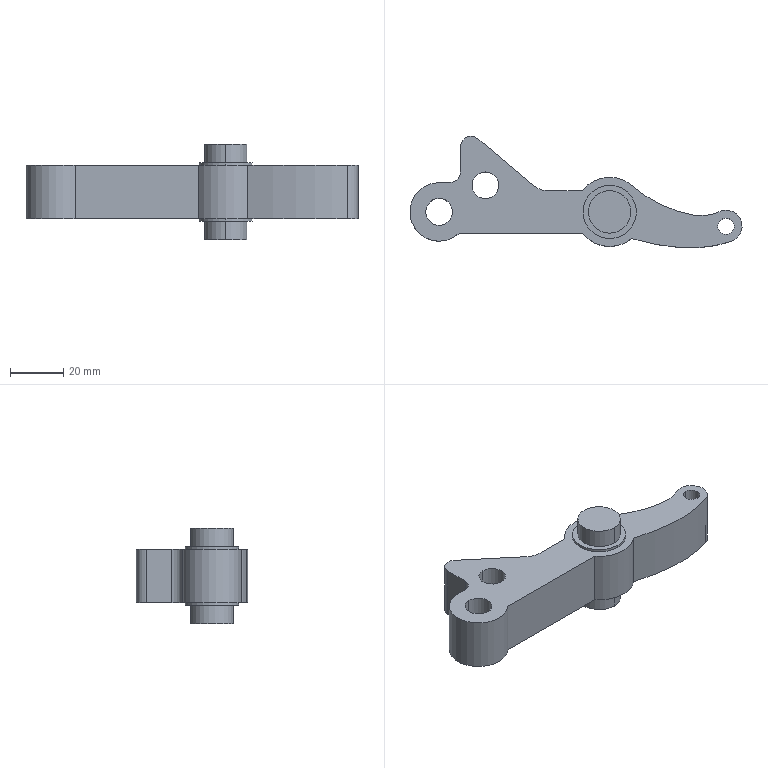Part | NX | features BREP 1 | 1 solid | 37 faces | box 124.672 x 41.892 x 36 mm | volume 48591 mm3 | cylinder 24 | plane 11 | spline 2 | commonest cylinder face diameters 15.96 x4 20 x4 8 x3 26 x3 6.1 x2 10.02 x2
STEP:
#1=CARTESIAN_POINT('',(-60.,156.98,-11.));
#2=VERTEX_POINT('',#1);
#3=CARTESIAN_POINT('',(-60.,141.02,-11.));
#4=VERTEX_POINT('',#3);
#5=CARTESIAN_POINT('',(-60.,149.,-11.));
#6=DIRECTION('',(0.,0.,-1.));
#7=DIRECTION('',(0.,1.,0.));
#8=AXIS2_PLACEMENT_3D('',#5,#6,#7);
#9=CIRCLE('',#8,7.98);
#10=EDGE_CURVE('',#2,#4,#9,.T.);
#11=ORIENTED_EDGE('',*,*,#10,.T.);
#12=CARTESIAN_POINT('',(-60.,141.02,-18.));
#13=VERTEX_POINT('',#12);
#14=CARTESIAN_POINT('',(-60.,141.02,18.));
#15=DIRECTION('',(0.,0.,1.));
#16=VECTOR('',#15,1000.);
#17=LINE('',#14,#16);
#18=EDGE_CURVE('',#13,#4,#17,.T.);
#19=ORIENTED_EDGE('',*,*,#18,.F.);
#20=CARTESIAN_POINT('',(-60.,156.98,-18.));
#21=VERTEX_POINT('',#20);
#22=CARTESIAN_POINT('',(-60.,149.,-18.));
#23=DIRECTION('',(0.,0.,1.));
#24=DIRECTION('',(0.,-1.,0.));
#25=AXIS2_PLACEMENT_3D('',#22,#23,#24);
#26=CIRCLE('',#25,7.98);
#27=EDGE_CURVE('',#13,#21,#26,.T.);
#28=ORIENTED_EDGE('',*,*,#27,.T.);
#29=CARTESIAN_POINT('',(-60.,156.98,18.));
#30=DIRECTION('',(0.,0.,-1.));
#31=VECTOR('',#30,1000.);
#32=LINE('',#29,#31);
#33=EDGE_CURVE('',#2,#21,#32,.T.);
#34=ORIENTED_EDGE('',*,*,#33,.F.);
#35=EDGE_LOOP('',(#11,#19,#28,#34));
#36=FACE_BOUND('',#35,.T.);
#37=CARTESIAN_POINT('',(-60.,149.,18.));
#38=DIRECTION('',(0.,0.,-1.));
#39=DIRECTION('',(0.,-1.,0.));
#40=AXIS2_PLACEMENT_3D('',#37,#38,#39);
#41=CYLINDRICAL_SURFACE('',#40,7.98);
#42=ADVANCED_FACE('',(#36),#41,.T.);
#43=CARTESIAN_POINT('',(-60.,139.,-11.));
#44=VERTEX_POINT('',#43);
#45=CARTESIAN_POINT('',(-60.,159.,-11.));
#46=VERTEX_POINT('',#45);
#47=CARTESIAN_POINT('',(-60.,149.,-11.));
#48=DIRECTION('',(0.,0.,1.));
#49=DIRECTION('',(0.,-1.,0.));
#50=AXIS2_PLACEMENT_3D('',#47,#48,#49);
#51=CIRCLE('',#50,10.);
#52=EDGE_CURVE('',#44,#46,#51,.T.);
#53=ORIENTED_EDGE('',*,*,#52,.T.);
#54=CARTESIAN_POINT('',(-60.,159.,-10.));
#55=VERTEX_POINT('',#54);
#56=CARTESIAN_POINT('',(-60.,159.,-11.));
#57=DIRECTION('',(0.,0.,-1.));
#58=VECTOR('',#57,1000.);
#59=LINE('',#56,#58);
#60=EDGE_CURVE('',#55,#46,#59,.T.);
#61=ORIENTED_EDGE('',*,*,#60,.F.);
#62=CARTESIAN_POINT('',(-60.,139.,-10.));
#63=VERTEX_POINT('',#62);
#64=CARTESIAN_POINT('',(-60.,149.,-10.));
#65=DIRECTION('',(0.,0.,1.));
#66=DIRECTION('',(0.,-1.,0.));
#67=AXIS2_PLACEMENT_3D('',#64,#65,#66);
#68=CIRCLE('',#67,10.);
#69=EDGE_CURVE('',#63,#55,#68,.T.);
#70=ORIENTED_EDGE('',*,*,#69,.F.);
#71=CARTESIAN_POINT('',(-60.,139.,-11.));
#72=DIRECTION('',(0.,0.,1.));
#73=VECTOR('',#72,1000.);
#74=LINE('',#71,#73);
#75=EDGE_CURVE('',#44,#63,#74,.T.);
#76=ORIENTED_EDGE('',*,*,#75,.F.);
#77=EDGE_LOOP('',(#53,#61,#70,#76));
#78=FACE_BOUND('',#77,.T.);
#79=CARTESIAN_POINT('',(-60.,149.,-11.));
#80=DIRECTION('',(0.,0.,1.));
#81=DIRECTION('',(0.,1.,0.));
#82=AXIS2_PLACEMENT_3D('',#79,#80,#81);
#83=CYLINDRICAL_SURFACE('',#82,10.);
#84=ADVANCED_FACE('',(#78),#83,.T.);
#85=CARTESIAN_POINT('',(-60.,141.02,18.));
#86=VERTEX_POINT('',#85);
#87=CARTESIAN_POINT('',(-60.,156.98,18.));
#88=VERTEX_POINT('',#87);
#89=CARTESIAN_POINT('',(-60.,149.,18.));
#90=DIRECTION('',(0.,0.,1.));
#91=DIRECTION('',(0.,-1.,0.));
#92=AXIS2_PLACEMENT_3D('',#89,#90,#91);
#93=CIRCLE('',#92,7.98);
#94=EDGE_CURVE('',#86,#88,#93,.T.);
#95=ORIENTED_EDGE('',*,*,#94,.F.);
#96=CARTESIAN_POINT('',(-60.,141.02,11.));
#97=VERTEX_POINT('',#96);
#98=CARTESIAN_POINT('',(-60.,141.02,18.));
#99=DIRECTION('',(0.,0.,-1.));
#100=VECTOR('',#99,1000.);
#101=LINE('',#98,#100);
#102=EDGE_CURVE('',#86,#97,#101,.T.);
#103=ORIENTED_EDGE('',*,*,#102,.T.);
#104=CARTESIAN_POINT('',(-60.,156.98,11.));
#105=VERTEX_POINT('',#104);
#106=CARTESIAN_POINT('',(-60.,149.,11.));
#107=DIRECTION('',(0.,0.,1.));
#108=DIRECTION('',(0.,-1.,0.));
#109=AXIS2_PLACEMENT_3D('',#106,#107,#108);
#110=CIRCLE('',#109,7.98);
#111=EDGE_CURVE('',#97,#105,#110,.T.);
#112=ORIENTED_EDGE('',*,*,#111,.T.);
#113=CARTESIAN_POINT('',(-60.,156.98,18.));
#114=DIRECTION('',(0.,0.,1.));
#115=VECTOR('',#114,1000.);
#116=LINE('',#113,#115);
#117=EDGE_CURVE('',#105,#88,#116,.T.);
#118=ORIENTED_EDGE('',*,*,#117,.T.);
#119=EDGE_LOOP('',(#95,#103,#112,#118));
#120=FACE_BOUND('',#119,.T.);
#121=CARTESIAN_POINT('',(-60.,149.,18.));
#122=DIRECTION('',(0.,0.,-1.));
#123=DIRECTION('',(0.,-1.,0.));
#124=AXIS2_PLACEMENT_3D('',#121,#122,#123);
#125=CYLINDRICAL_SURFACE('',#124,7.98);
#126=ADVANCED_FACE('',(#120),#125,.T.);
#127=CARTESIAN_POINT('',(-60.,139.,11.));
#128=VERTEX_POINT('',#127);
#129=CARTESIAN_POINT('',(-60.,159.,11.));
#130=VERTEX_POINT('',#129);
#131=CARTESIAN_POINT('',(-60.,149.,11.));
#132=DIRECTION('',(0.,0.,1.));
#133=DIRECTION('',(0.,-1.,0.));
#134=AXIS2_PLACEMENT_3D('',#131,#132,#133);
#135=CIRCLE('',#134,10.);
#136=EDGE_CURVE('',#128,#130,#135,.T.);
#137=ORIENTED_EDGE('',*,*,#136,.F.);
#138=CARTESIAN_POINT('',(-60.,139.,10.));
#139=VERTEX_POINT('',#138);
#140=CARTESIAN_POINT('',(-60.,139.,11.));
#141=DIRECTION('',(0.,0.,-1.));
#142=VECTOR('',#141,1000.);
#143=LINE('',#140,#142);
#144=EDGE_CURVE('',#128,#139,#143,.T.);
#145=ORIENTED_EDGE('',*,*,#144,.T.);
#146=CARTESIAN_POINT('',(-60.,159.,10.));
#147=VERTEX_POINT('',#146);
#148=CARTESIAN_POINT('',(-60.,149.,10.));
#149=DIRECTION('',(0.,0.,1.));
#150=DIRECTION('',(0.,-1.,0.));
#151=AXIS2_PLACEMENT_3D('',#148,#149,#150);
#152=CIRCLE('',#151,10.);
#153=EDGE_CURVE('',#139,#147,#152,.T.);
#154=ORIENTED_EDGE('',*,*,#153,.T.);
#155=CARTESIAN_POINT('',(-60.,159.,11.));
#156=DIRECTION('',(0.,0.,1.));
#157=VECTOR('',#156,1000.);
#158=LINE('',#155,#157);
#159=EDGE_CURVE('',#147,#130,#158,.T.);
#160=ORIENTED_EDGE('',*,*,#159,.T.);
#161=EDGE_LOOP('',(#137,#145,#154,#160));
#162=FACE_BOUND('',#161,.T.);
#163=CARTESIAN_POINT('',(-60.,149.,11.));
#164=DIRECTION('',(0.,0.,-1.));
#165=DIRECTION('',(0.,-1.,0.));
#166=AXIS2_PLACEMENT_3D('',#163,#164,#165);
#167=CYLINDRICAL_SURFACE('',#166,10.);
#168=ADVANCED_FACE('',(#162),#167,.T.);
#169=CARTESIAN_POINT('',(-112.,177.388,10.));
#170=VERTEX_POINT('',#169);
#171=CARTESIAN_POINT('',(-116.,173.388,10.));
#172=VERTEX_POINT('',#171);
#173=CARTESIAN_POINT('',(-112.,173.388,10.));
#174=DIRECTION('',(0.,0.,1.));
#175=DIRECTION('',(0.,-1.,0.));
#176=AXIS2_PLACEMENT_3D('',#173,#174,#175);
#177=CIRCLE('',#176,4.);
#178=EDGE_CURVE('',#170,#172,#177,.T.);
#179=ORIENTED_EDGE('',*,*,#178,.F.);
#180=CARTESIAN_POINT('',(-112.,177.388,-10.));
#181=VERTEX_POINT('',#180);
#182=CARTESIAN_POINT('',(-112.,177.388,10.));
#183=DIRECTION('',(0.,0.,-1.));
#184=VECTOR('',#183,1000.);
#185=LINE('',#182,#184);
#186=EDGE_CURVE('',#170,#181,#185,.T.);
#187=ORIENTED_EDGE('',*,*,#186,.T.);
#188=CARTESIAN_POINT('',(-116.,173.388,-10.));
#189=VERTEX_POINT('',#188);
#190=CARTESIAN_POINT('',(-112.,173.388,-10.));
#191=DIRECTION('',(0.,0.,-1.));
#192=DIRECTION('',(0.,-1.,0.));
#193=AXIS2_PLACEMENT_3D('',#190,#191,#192);
#194=CIRCLE('',#193,4.);
#195=EDGE_CURVE('',#189,#181,#194,.T.);
#196=ORIENTED_EDGE('',*,*,#195,.F.);
#197=CARTESIAN_POINT('',(-116.,173.388,10.));
#198=DIRECTION('',(0.,0.,-1.));
#199=VECTOR('',#198,1000.);
#200=LINE('',#197,#199);
#201=EDGE_CURVE('',#172,#189,#200,.T.);
#202=ORIENTED_EDGE('',*,*,#201,.F.);
#203=EDGE_LOOP('',(#179,#187,#196,#202));
#204=FACE_BOUND('',#203,.T.);
#205=CARTESIAN_POINT('',(-112.,173.388,10.));
#206=DIRECTION('',(0.,0.,-1.));
#207=DIRECTION('',(0.,-1.,0.));
#208=AXIS2_PLACEMENT_3D('',#205,#206,#207);
#209=CYLINDRICAL_SURFACE('',#208,4.);
#210=ADVANCED_FACE('',(#204),#209,.T.);
#211=CARTESIAN_POINT('',(-16.328,146.688,10.));
#212=VERTEX_POINT('',#211);
#213=CARTESIAN_POINT('',(-16.328,140.588,10.));
#214=VERTEX_POINT('',#213);
#215=CARTESIAN_POINT('',(-16.328,143.638,10.));
#216=DIRECTION('',(0.,0.,1.));
#217=DIRECTION('',(0.,1.,0.));
#218=AXIS2_PLACEMENT_3D('',#215,#216,#217);
#219=CIRCLE('',#218,3.05);
#220=EDGE_CURVE('',#212,#214,#219,.T.);
#221=ORIENTED_EDGE('',*,*,#220,.T.);
#222=CARTESIAN_POINT('',(-16.328,140.588,-10.));
#223=VERTEX_POINT('',#222);
#224=CARTESIAN_POINT('',(-16.328,140.588,10.));
#225=DIRECTION('',(0.,0.,-1.));
#226=VECTOR('',#225,1000.);
#227=LINE('',#224,#226);
#228=EDGE_CURVE('',#214,#223,#227,.T.);
#229=ORIENTED_EDGE('',*,*,#228,.T.);
#230=CARTESIAN_POINT('',(-16.328,146.688,-10.));
#231=VERTEX_POINT('',#230);
#232=CARTESIAN_POINT('',(-16.328,143.638,-10.));
#233=DIRECTION('',(0.,0.,1.));
#234=DIRECTION('',(0.,1.,0.));
#235=AXIS2_PLACEMENT_3D('',#232,#233,#234);
#236=CIRCLE('',#235,3.05);
#237=EDGE_CURVE('',#231,#223,#236,.T.);
#238=ORIENTED_EDGE('',*,*,#237,.F.);
#239=CARTESIAN_POINT('',(-16.328,146.688,10.));
#240=DIRECTION('',(0.,0.,1.));
#241=VECTOR('',#240,1000.);
#242=LINE('',#239,#241);
#243=EDGE_CURVE('',#231,#212,#242,.T.);
#244=ORIENTED_EDGE('',*,*,#243,.T.);
#245=EDGE_LOOP('',(#221,#229,#238,#244));
#246=FACE_BOUND('',#245,.T.);
#247=CARTESIAN_POINT('',(-16.328,143.638,10.));
#248=DIRECTION('',(0.,0.,-1.));
#249=DIRECTION('',(0.,-1.,0.));
#250=AXIS2_PLACEMENT_3D('',#247,#248,#249);
#251=CYLINDRICAL_SURFACE('',#250,3.05);
#252=ADVANCED_FACE('',(#246),#251,.F.);
#253=CARTESIAN_POINT('',(-16.328,149.638,10.));
#254=VERTEX_POINT('',#253);
#255=CARTESIAN_POINT('',(-19.02,149.,10.));
#256=VERTEX_POINT('',#255);
#257=CARTESIAN_POINT('',(-16.328,143.638,10.));
#258=DIRECTION('',(0.,0.,1.));
#259=DIRECTION('',(0.,1.,0.));
#260=AXIS2_PLACEMENT_3D('',#257,#258,#259);
#261=CIRCLE('',#260,6.);
#262=EDGE_CURVE('',#254,#256,#261,.T.);
#263=ORIENTED_EDGE('',*,*,#262,.F.);
#264=CARTESIAN_POINT('',(-16.328,149.638,-10.));
#265=VERTEX_POINT('',#264);
#266=CARTESIAN_POINT('',(-16.328,149.638,10.));
#267=DIRECTION('',(0.,0.,-1.));
#268=VECTOR('',#267,1000.);
#269=LINE('',#266,#268);
#270=EDGE_CURVE('',#254,#265,#269,.T.);
#271=ORIENTED_EDGE('',*,*,#270,.T.);
#272=CARTESIAN_POINT('',(-19.02,149.,-10.));
#273=VERTEX_POINT('',#272);
#274=CARTESIAN_POINT('',(-16.328,143.638,-10.));
#275=DIRECTION('',(0.,0.,1.));
#276=DIRECTION('',(0.,1.,0.));
#277=AXIS2_PLACEMENT_3D('',#274,#275,#276);
#278=CIRCLE('',#277,6.);
#279=EDGE_CURVE('',#265,#273,#278,.T.);
#280=ORIENTED_EDGE('',*,*,#279,.T.);
#281=CARTESIAN_POINT('',(-19.02,149.,10.));
#282=DIRECTION('',(0.,0.,-1.));
#283=VECTOR('',#282,1000.);
#284=LINE('',#281,#283);
#285=EDGE_CURVE('',#256,#273,#284,.T.);
#286=ORIENTED_EDGE('',*,*,#285,.F.);
#287=EDGE_LOOP('',(#263,#271,#280,#286));
#288=FACE_BOUND('',#287,.T.);
#289=CARTESIAN_POINT('',(-16.328,143.638,10.));
#290=DIRECTION('',(0.,0.,-1.));
#291=DIRECTION('',(0.,-1.,0.));
#292=AXIS2_PLACEMENT_3D('',#289,#290,#291);
#293=CYLINDRICAL_SURFACE('',#292,6.);
#294=ADVANCED_FACE('',(#288),#293,.T.);
#295=CARTESIAN_POINT('',(-106.679,164.01,10.));
#296=VERTEX_POINT('',#295);
#297=CARTESIAN_POINT('',(-106.679,153.99,10.));
#298=VERTEX_POINT('',#297);
#299=CARTESIAN_POINT('',(-106.679,159.,10.));
#300=DIRECTION('',(0.,0.,1.));
#301=DIRECTION('',(0.,-1.,0.));
#302=AXIS2_PLACEMENT_3D('',#299,#300,#301);
#303=CIRCLE('',#302,5.01);
#304=EDGE_CURVE('',#296,#298,#303,.T.);
#305=ORIENTED_EDGE('',*,*,#304,.T.);
#306=CARTESIAN_POINT('',(-106.679,153.99,-10.));
#307=VERTEX_POINT('',#306);
#308=CARTESIAN_POINT('',(-106.679,153.99,10.));
#309=DIRECTION('',(0.,0.,1.));
#310=VECTOR('',#309,1000.);
#311=LINE('',#308,#310);
#312=EDGE_CURVE('',#307,#298,#311,.T.);
#313=ORIENTED_EDGE('',*,*,#312,.F.);
#314=CARTESIAN_POINT('',(-106.679,164.01,-10.));
#315=VERTEX_POINT('',#314);
#316=CARTESIAN_POINT('',(-106.679,159.,-10.));
#317=DIRECTION('',(0.,0.,1.));
#318=DIRECTION('',(0.,-1.,0.));
#319=AXIS2_PLACEMENT_3D('',#316,#317,#318);
#320=CIRCLE('',#319,5.01);
#321=EDGE_CURVE('',#315,#307,#320,.T.);
#322=ORIENTED_EDGE('',*,*,#321,.F.);
#323=CARTESIAN_POINT('',(-106.679,164.01,10.));
#324=DIRECTION('',(0.,0.,-1.));
#325=VECTOR('',#324,1000.);
#326=LINE('',#323,#325);
#327=EDGE_CURVE('',#296,#315,#326,.T.);
#328=ORIENTED_EDGE('',*,*,#327,.F.);
#329=EDGE_LOOP('',(#305,#313,#322,#328));
#330=FACE_BOUND('',#329,.T.);
#331=CARTESIAN_POINT('',(-106.679,159.,10.));
#332=DIRECTION('',(0.,0.,-1.));
#333=DIRECTION('',(0.,-1.,0.));
#334=AXIS2_PLACEMENT_3D('',#331,#332,#333);
#335=CYLINDRICAL_SURFACE('',#334,5.01);
#336=ADVANCED_FACE('',(#330),#335,.F.);
#337=CARTESIAN_POINT('',(-124.,154.05,10.));
#338=VERTEX_POINT('',#337);
#339=CARTESIAN_POINT('',(-124.,143.95,10.));
#340=VERTEX_POINT('',#339);
#341=CARTESIAN_POINT('',(-124.,149.,10.));
#342=DIRECTION('',(0.,0.,1.));
#343=DIRECTION('',(0.,-1.,0.));
#344=AXIS2_PLACEMENT_3D('',#341,#342,#343);
#345=CIRCLE('',#344,5.05);
#346=EDGE_CURVE('',#338,#340,#345,.T.);
#347=ORIENTED_EDGE('',*,*,#346,.T.);
#348=CARTESIAN_POINT('',(-124.,143.95,-10.));
#349=VERTEX_POINT('',#348);
#350=CARTESIAN_POINT('',(-124.,143.95,10.));
#351=DIRECTION('',(0.,0.,-1.));
#352=VECTOR('',#351,1000.);
#353=LINE('',#350,#352);
#354=EDGE_CURVE('',#340,#349,#353,.T.);
#355=ORIENTED_EDGE('',*,*,#354,.T.);
#356=CARTESIAN_POINT('',(-124.,154.05,-10.));
#357=VERTEX_POINT('',#356);
#358=CARTESIAN_POINT('',(-124.,149.,-10.));
#359=DIRECTION('',(0.,0.,1.));
#360=DIRECTION('',(0.,-1.,0.));
#361=AXIS2_PLACEMENT_3D('',#358,#359,#360);
#362=CIRCLE('',#361,5.05);
#363=EDGE_CURVE('',#357,#349,#362,.T.);
#364=ORIENTED_EDGE('',*,*,#363,.F.);
#365=CARTESIAN_POINT('',(-124.,154.05,10.));
#366=DIRECTION('',(0.,0.,1.));
#367=VECTOR('',#366,1000.);
#368=LINE('',#365,#367);
#369=EDGE_CURVE('',#357,#338,#368,.T.);
#370=ORIENTED_EDGE('',*,*,#369,.T.);
#371=EDGE_LOOP('',(#347,#355,#364,#370));
#372=FACE_BOUND('',#371,.T.);
#373=CARTESIAN_POINT('',(-124.,149.,10.));
#374=DIRECTION('',(0.,0.,-1.));
#375=DIRECTION('',(0.,-1.,0.));
#376=AXIS2_PLACEMENT_3D('',#373,#374,#375);
#377=CYLINDRICAL_SURFACE('',#376,5.05);
#378=ADVANCED_FACE('',(#372),#377,.F.);
#379=CARTESIAN_POINT('',(-60.,162.,10.));
#380=VERTEX_POINT('',#379);
#381=CARTESIAN_POINT('',(-70.247,157.,10.));
#382=VERTEX_POINT('',#381);
#383=CARTESIAN_POINT('',(-60.,149.,10.));
#384=DIRECTION('',(0.,0.,1.));
#385=DIRECTION('',(0.,-1.,0.));
#386=AXIS2_PLACEMENT_3D('',#383,#384,#385);
#387=CIRCLE('',#386,13.);
#388=EDGE_CURVE('',#380,#382,#387,.T.);
#389=ORIENTED_EDGE('',*,*,#388,.F.);
#390=CARTESIAN_POINT('',(-60.,162.,-10.));
#391=VERTEX_POINT('',#390);
#392=CARTESIAN_POINT('',(-60.,162.,10.));
#393=DIRECTION('',(0.,0.,-1.));
#394=VECTOR('',#393,1000.);
#395=LINE('',#392,#394);
#396=EDGE_CURVE('',#380,#391,#395,.T.);
#397=ORIENTED_EDGE('',*,*,#396,.T.);
#398=CARTESIAN_POINT('',(-70.247,157.,-10.));
#399=VERTEX_POINT('',#398);
#400=CARTESIAN_POINT('',(-60.,149.,-10.));
#401=DIRECTION('',(0.,0.,1.));
#402=DIRECTION('',(0.,-1.,0.));
#403=AXIS2_PLACEMENT_3D('',#400,#401,#402);
#404=CIRCLE('',#403,13.);
#405=EDGE_CURVE('',#391,#399,#404,.T.);
#406=ORIENTED_EDGE('',*,*,#405,.T.);
#407=CARTESIAN_POINT('',(-70.247,157.,10.));
#408=DIRECTION('',(0.,0.,-1.));
#409=VECTOR('',#408,1000.);
#410=LINE('',#407,#409);
#411=EDGE_CURVE('',#382,#399,#410,.T.);
#412=ORIENTED_EDGE('',*,*,#411,.F.);
#413=EDGE_LOOP('',(#389,#397,#406,#412));
#414=FACE_BOUND('',#413,.T.);
#415=CARTESIAN_POINT('',(-60.,149.,10.));
#416=DIRECTION('',(0.,0.,-1.));
#417=DIRECTION('',(0.,-1.,0.));
#418=AXIS2_PLACEMENT_3D('',#415,#416,#417);
#419=CYLINDRICAL_SURFACE('',#418,13.);
#420=ADVANCED_FACE('',(#414),#419,.T.);
#421=CARTESIAN_POINT('',(-51.681,139.01,10.));
#422=VERTEX_POINT('',#421);
#423=CARTESIAN_POINT('',(-51.681,139.01,-10.));
#424=VERTEX_POINT('',#423);
#425=CARTESIAN_POINT('',(-51.681,139.01,10.));
#426=DIRECTION('',(0.,0.,-1.));
#427=VECTOR('',#426,1000.);
#428=LINE('',#425,#427);
#429=EDGE_CURVE('',#422,#424,#428,.T.);
#430=ORIENTED_EDGE('',*,*,#429,.F.);
#431=CARTESIAN_POINT('',(-70.247,141.,10.));
#432=VERTEX_POINT('',#431);
#433=CARTESIAN_POINT('',(-60.,149.,10.));
#434=DIRECTION('',(0.,0.,1.));
#435=DIRECTION('',(0.,-1.,0.));
#436=AXIS2_PLACEMENT_3D('',#433,#434,#435);
#437=CIRCLE('',#436,13.);
#438=EDGE_CURVE('',#432,#422,#437,.T.);
#439=ORIENTED_EDGE('',*,*,#438,.F.);
#440=CARTESIAN_POINT('',(-70.247,141.,-10.));
#441=VERTEX_POINT('',#440);
#442=CARTESIAN_POINT('',(-70.247,141.,10.));
#443=DIRECTION('',(0.,0.,-1.));
#444=VECTOR('',#443,1000.);
#445=LINE('',#442,#444);
#446=EDGE_CURVE('',#432,#441,#445,.T.);
#447=ORIENTED_EDGE('',*,*,#446,.T.);
#448=CARTESIAN_POINT('',(-60.,149.,-10.));
#449=DIRECTION('',(0.,0.,1.));
#450=DIRECTION('',(0.,-1.,0.));
#451=AXIS2_PLACEMENT_3D('',#448,#449,#450);
#452=CIRCLE('',#451,13.);
#453=EDGE_CURVE('',#441,#424,#452,.T.);
#454=ORIENTED_EDGE('',*,*,#453,.T.);
#455=EDGE_LOOP('',(#430,#439,#447,#454));
#456=FACE_BOUND('',#455,.T.);
#457=CARTESIAN_POINT('',(-60.,149.,10.));
#458=DIRECTION('',(0.,0.,-1.));
#459=DIRECTION('',(0.,-1.,0.));
#460=AXIS2_PLACEMENT_3D('',#457,#458,#459);
#461=CYLINDRICAL_SURFACE('',#460,13.);
#462=ADVANCED_FACE('',(#456),#461,.T.);
#463=CARTESIAN_POINT('',(-60.,149.,10.));
#464=DIRECTION('',(0.,0.,1.));
#465=DIRECTION('',(0.,-1.,0.));
#466=AXIS2_PLACEMENT_3D('',#463,#464,#465);
#467=CIRCLE('',#466,10.);
#468=EDGE_CURVE('',#147,#139,#467,.T.);
#469=ORIENTED_EDGE('',*,*,#468,.F.);
#470=ORIENTED_EDGE('',*,*,#153,.F.);
#471=EDGE_LOOP('',(#469,#470));
#472=FACE_BOUND('',#471,.T.);
#473=ORIENTED_EDGE('',*,*,#346,.F.);
#474=CARTESIAN_POINT('',(-124.,149.,10.));
#475=DIRECTION('',(0.,0.,1.));
#476=DIRECTION('',(0.,-1.,0.));
#477=AXIS2_PLACEMENT_3D('',#474,#475,#476);
#478=CIRCLE('',#477,5.05);
#479=EDGE_CURVE('',#340,#338,#478,.T.);
#480=ORIENTED_EDGE('',*,*,#479,.F.);
#481=EDGE_LOOP('',(#473,#480));
#482=FACE_BOUND('',#481,.T.);
#483=CARTESIAN_POINT('',(-88.477,158.872,10.));
#484=VERTEX_POINT('',#483);
#485=CARTESIAN_POINT('',(-109.429,176.452,10.));
#486=VERTEX_POINT('',#485);
#487=CARTESIAN_POINT('',(-86.247,157.,10.));
#488=DIRECTION('',(-0.766,0.6428,0.));
#489=VECTOR('',#488,1000.);
#490=LINE('',#487,#489);
#491=EDGE_CURVE('',#484,#486,#490,.T.);
#492=ORIENTED_EDGE('',*,*,#491,.T.);
#493=CARTESIAN_POINT('',(-112.,173.388,10.));
#494=DIRECTION('',(0.,0.,1.));
#495=DIRECTION('',(0.,-1.,0.));
#496=AXIS2_PLACEMENT_3D('',#493,#494,#495);
#497=CIRCLE('',#496,4.);
#498=EDGE_CURVE('',#486,#170,#497,.T.);
#499=ORIENTED_EDGE('',*,*,#498,.T.);
#500=ORIENTED_EDGE('',*,*,#178,.T.);
#501=CARTESIAN_POINT('',(-116.,164.,10.));
#502=VERTEX_POINT('',#501);
#503=CARTESIAN_POINT('',(-116.,181.966,10.));
#504=DIRECTION('',(0.,-1.,0.));
#505=VECTOR('',#504,1000.);
#506=LINE('',#503,#505);
#507=EDGE_CURVE('',#172,#502,#506,.T.);
#508=ORIENTED_EDGE('',*,*,#507,.T.);
#509=CARTESIAN_POINT('',(-120.,160.,10.));
#510=VERTEX_POINT('',#509);
#511=CARTESIAN_POINT('',(-120.,164.,10.));
#512=DIRECTION('',(0.,0.,-1.));
#513=DIRECTION('',(0.,-1.,0.));
#514=AXIS2_PLACEMENT_3D('',#511,#512,#513);
#515=CIRCLE('',#514,4.);
#516=EDGE_CURVE('',#502,#510,#515,.T.);
#517=ORIENTED_EDGE('',*,*,#516,.T.);
#518=CARTESIAN_POINT('',(-124.,160.,10.));
#519=VERTEX_POINT('',#518);
#520=CARTESIAN_POINT('',(-124.,160.,10.));
#521=DIRECTION('',(-1.,0.,0.));
#522=VECTOR('',#521,1000.);
#523=LINE('',#520,#522);
#524=EDGE_CURVE('',#510,#519,#523,.T.);
#525=ORIENTED_EDGE('',*,*,#524,.T.);
#526=CARTESIAN_POINT('',(-116.45,141.,10.));
#527=VERTEX_POINT('',#526);
#528=CARTESIAN_POINT('',(-124.,149.,10.));
#529=DIRECTION('',(0.,0.,1.));
#530=DIRECTION('',(0.,-1.,0.));
#531=AXIS2_PLACEMENT_3D('',#528,#529,#530);
#532=CIRCLE('',#531,11.);
#533=EDGE_CURVE('',#519,#527,#532,.T.);
#534=ORIENTED_EDGE('',*,*,#533,.T.);
#535=CARTESIAN_POINT('',(-70.247,141.,10.));
#536=DIRECTION('',(1.,0.,0.));
#537=VECTOR('',#536,1000.);
#538=LINE('',#535,#537);
#539=EDGE_CURVE('',#527,#432,#538,.T.);
#540=ORIENTED_EDGE('',*,*,#539,.T.);
#541=ORIENTED_EDGE('',*,*,#438,.T.);
#542=CARTESIAN_POINT('',(-14.301,137.991,10.));
#543=VERTEX_POINT('',#542);
#544=CARTESIAN_POINT('',(-51.681,139.01,10.));
#545=CARTESIAN_POINT('',(-29.498,132.535,10.));
#546=CARTESIAN_POINT('',(-14.301,137.991,10.));
#547=B_SPLINE_CURVE_WITH_KNOTS('',2,(#544,#545,#546),.UNSPECIFIED.,.F.,.F.,(3,3),(0.,1.),.PIECEWISE_BEZIER_KNOTS.);
#548=EDGE_CURVE('',#422,#543,#547,.T.);
#549=ORIENTED_EDGE('',*,*,#548,.T.);
#550=CARTESIAN_POINT('',(-16.328,143.638,10.));
#551=DIRECTION('',(0.,0.,1.));
#552=DIRECTION('',(0.,1.,0.));
#553=AXIS2_PLACEMENT_3D('',#550,#551,#552);
#554=CIRCLE('',#553,6.);
#555=EDGE_CURVE('',#543,#254,#554,.T.);
#556=ORIENTED_EDGE('',*,*,#555,.T.);
#557=ORIENTED_EDGE('',*,*,#262,.T.);
#558=CARTESIAN_POINT('',(-51.067,158.444,10.));
#559=VERTEX_POINT('',#558);
#560=CARTESIAN_POINT('',(-51.067,158.444,10.));
#561=CARTESIAN_POINT('',(-45.43,153.113,10.));
#562=CARTESIAN_POINT('',(-28.567,144.208,10.));
#563=CARTESIAN_POINT('',(-19.02,149.,10.));
#564=B_SPLINE_CURVE_WITH_KNOTS('',3,(#560,#561,#562,#563),.UNSPECIFIED.,.F.,.F.,(4,4),(0.,1.),.PIECEWISE_BEZIER_KNOTS.);
#565=EDGE_CURVE('',#559,#256,#564,.T.);
#566=ORIENTED_EDGE('',*,*,#565,.F.);
#567=CARTESIAN_POINT('',(-60.,149.,10.));
#568=DIRECTION('',(0.,0.,1.));
#569=DIRECTION('',(0.,-1.,0.));
#570=AXIS2_PLACEMENT_3D('',#567,#568,#569);
#571=CIRCLE('',#570,13.);
#572=EDGE_CURVE('',#559,#380,#571,.T.);
#573=ORIENTED_EDGE('',*,*,#572,.T.);
#574=ORIENTED_EDGE('',*,*,#388,.T.);
#575=CARTESIAN_POINT('',(-83.335,157.,10.));
#576=VERTEX_POINT('',#575);
#577=CARTESIAN_POINT('',(-70.247,157.,10.));
#578=DIRECTION('',(-1.,0.,0.));
#579=VECTOR('',#578,1000.);
#580=LINE('',#577,#579);
#581=EDGE_CURVE('',#382,#576,#580,.T.);
#582=ORIENTED_EDGE('',*,*,#581,.T.);
#583=CARTESIAN_POINT('',(-83.335,165.,10.));
#584=DIRECTION('',(0.,0.,-1.));
#585=DIRECTION('',(0.,-1.,0.));
#586=AXIS2_PLACEMENT_3D('',#583,#584,#585);
#587=CIRCLE('',#586,8.);
#588=EDGE_CURVE('',#576,#484,#587,.T.);
#589=ORIENTED_EDGE('',*,*,#588,.T.);
#590=EDGE_LOOP('',(#492,#499,#500,#508,#517,#525,#534,#540,#541,#549,#556,#557,#566,#573,#574,#582,#589));
#591=FACE_BOUND('',#590,.T.);
#592=ORIENTED_EDGE('',*,*,#304,.F.);
#593=CARTESIAN_POINT('',(-106.679,159.,10.));
#594=DIRECTION('',(0.,0.,1.));
#595=DIRECTION('',(0.,-1.,0.));
#596=AXIS2_PLACEMENT_3D('',#593,#594,#595);
#597=CIRCLE('',#596,5.01);
#598=EDGE_CURVE('',#298,#296,#597,.T.);
#599=ORIENTED_EDGE('',*,*,#598,.F.);
#600=EDGE_LOOP('',(#592,#599));
#601=FACE_BOUND('',#600,.T.);
#602=ORIENTED_EDGE('',*,*,#220,.F.);
#603=CARTESIAN_POINT('',(-16.328,143.638,10.));
#604=DIRECTION('',(0.,0.,1.));
#605=DIRECTION('',(0.,1.,0.));
#606=AXIS2_PLACEMENT_3D('',#603,#604,#605);
#607=CIRCLE('',#606,3.05);
#608=EDGE_CURVE('',#214,#212,#607,.T.);
#609=ORIENTED_EDGE('',*,*,#608,.F.);
#610=EDGE_LOOP('',(#602,#609));
#611=FACE_BOUND('',#610,.T.);
#612=CARTESIAN_POINT('',(-60.,149.,10.));
#613=DIRECTION('',(0.,0.,1.));
#614=DIRECTION('',(0.,1.,0.));
#615=AXIS2_PLACEMENT_3D('',#612,#613,#614);
#616=PLANE('',#615);
#617=ADVANCED_FACE('',(#472,#482,#591,#601,#611),#616,.T.);
#618=ORIENTED_EDGE('',*,*,#69,.T.);
#619=CARTESIAN_POINT('',(-60.,149.,-10.));
#620=DIRECTION('',(0.,0.,1.));
#621=DIRECTION('',(0.,-1.,0.));
#622=AXIS2_PLACEMENT_3D('',#619,#620,#621);
#623=CIRCLE('',#622,10.);
#624=EDGE_CURVE('',#55,#63,#623,.T.);
#625=ORIENTED_EDGE('',*,*,#624,.T.);
#626=EDGE_LOOP('',(#618,#625));
#627=FACE_BOUND('',#626,.T.);
#628=CARTESIAN_POINT('',(-116.,164.,-10.));
#629=VERTEX_POINT('',#628);
#630=CARTESIAN_POINT('',(-116.,181.966,-10.));
#631=DIRECTION('',(0.,-1.,0.));
#632=VECTOR('',#631,1000.);
#633=LINE('',#630,#632);
#634=EDGE_CURVE('',#189,#629,#633,.T.);
#635=ORIENTED_EDGE('',*,*,#634,.F.);
#636=ORIENTED_EDGE('',*,*,#195,.T.);
#637=CARTESIAN_POINT('',(-109.429,176.452,-10.));
#638=VERTEX_POINT('',#637);
#639=CARTESIAN_POINT('',(-112.,173.388,-10.));
#640=DIRECTION('',(0.,0.,-1.));
#641=DIRECTION('',(0.,-1.,0.));
#642=AXIS2_PLACEMENT_3D('',#639,#640,#641);
#643=CIRCLE('',#642,4.);
#644=EDGE_CURVE('',#181,#638,#643,.T.);
#645=ORIENTED_EDGE('',*,*,#644,.T.);
#646=CARTESIAN_POINT('',(-88.477,158.872,-10.));
#647=VERTEX_POINT('',#646);
#648=CARTESIAN_POINT('',(-86.247,157.,-10.));
#649=DIRECTION('',(-0.766,0.6428,0.));
#650=VECTOR('',#649,1000.);
#651=LINE('',#648,#650);
#652=EDGE_CURVE('',#647,#638,#651,.T.);
#653=ORIENTED_EDGE('',*,*,#652,.F.);
#654=CARTESIAN_POINT('',(-83.335,157.,-10.));
#655=VERTEX_POINT('',#654);
#656=CARTESIAN_POINT('',(-83.335,165.,-10.));
#657=DIRECTION('',(0.,0.,1.));
#658=DIRECTION('',(0.,-1.,0.));
#659=AXIS2_PLACEMENT_3D('',#656,#657,#658);
#660=CIRCLE('',#659,8.);
#661=EDGE_CURVE('',#647,#655,#660,.T.);
#662=ORIENTED_EDGE('',*,*,#661,.T.);
#663=CARTESIAN_POINT('',(-70.247,157.,-10.));
#664=DIRECTION('',(-1.,0.,0.));
#665=VECTOR('',#664,1000.);
#666=LINE('',#663,#665);
#667=EDGE_CURVE('',#399,#655,#666,.T.);
#668=ORIENTED_EDGE('',*,*,#667,.F.);
#669=ORIENTED_EDGE('',*,*,#405,.F.);
#670=CARTESIAN_POINT('',(-51.067,158.444,-10.));
#671=VERTEX_POINT('',#670);
#672=CARTESIAN_POINT('',(-60.,149.,-10.));
#673=DIRECTION('',(0.,0.,1.));
#674=DIRECTION('',(0.,-1.,0.));
#675=AXIS2_PLACEMENT_3D('',#672,#673,#674);
#676=CIRCLE('',#675,13.);
#677=EDGE_CURVE('',#671,#391,#676,.T.);
#678=ORIENTED_EDGE('',*,*,#677,.F.);
#679=CARTESIAN_POINT('',(-51.067,158.444,-10.));
#680=CARTESIAN_POINT('',(-45.43,153.113,-10.));
#681=CARTESIAN_POINT('',(-28.567,144.208,-10.));
#682=CARTESIAN_POINT('',(-19.02,149.,-10.));
#683=B_SPLINE_CURVE_WITH_KNOTS('',3,(#679,#680,#681,#682),.UNSPECIFIED.,.F.,.F.,(4,4),(0.,1.),.PIECEWISE_BEZIER_KNOTS.);
#684=EDGE_CURVE('',#671,#273,#683,.T.);
#685=ORIENTED_EDGE('',*,*,#684,.T.);
#686=ORIENTED_EDGE('',*,*,#279,.F.);
#687=CARTESIAN_POINT('',(-14.301,137.991,-10.));
#688=VERTEX_POINT('',#687);
#689=CARTESIAN_POINT('',(-16.328,143.638,-10.));
#690=DIRECTION('',(0.,0.,1.));
#691=DIRECTION('',(0.,1.,0.));
#692=AXIS2_PLACEMENT_3D('',#689,#690,#691);
#693=CIRCLE('',#692,6.);
#694=EDGE_CURVE('',#688,#265,#693,.T.);
#695=ORIENTED_EDGE('',*,*,#694,.F.);
#696=CARTESIAN_POINT('',(-51.681,139.01,-10.));
#697=CARTESIAN_POINT('',(-29.498,132.535,-10.));
#698=CARTESIAN_POINT('',(-14.301,137.991,-10.));
#699=B_SPLINE_CURVE_WITH_KNOTS('',2,(#696,#697,#698),.UNSPECIFIED.,.F.,.F.,(3,3),(0.,1.),.PIECEWISE_BEZIER_KNOTS.);
#700=EDGE_CURVE('',#424,#688,#699,.T.);
#701=ORIENTED_EDGE('',*,*,#700,.F.);
#702=ORIENTED_EDGE('',*,*,#453,.F.);
#703=CARTESIAN_POINT('',(-116.45,141.,-10.));
#704=VERTEX_POINT('',#703);
#705=CARTESIAN_POINT('',(-70.247,141.,-10.));
#706=DIRECTION('',(1.,0.,0.));
#707=VECTOR('',#706,1000.);
#708=LINE('',#705,#707);
#709=EDGE_CURVE('',#704,#441,#708,.T.);
#710=ORIENTED_EDGE('',*,*,#709,.F.);
#711=CARTESIAN_POINT('',(-124.,160.,-10.));
#712=VERTEX_POINT('',#711);
#713=CARTESIAN_POINT('',(-124.,149.,-10.));
#714=DIRECTION('',(0.,0.,1.));
#715=DIRECTION('',(0.,-1.,0.));
#716=AXIS2_PLACEMENT_3D('',#713,#714,#715);
#717=CIRCLE('',#716,11.);
#718=EDGE_CURVE('',#712,#704,#717,.T.);
#719=ORIENTED_EDGE('',*,*,#718,.F.);
#720=CARTESIAN_POINT('',(-120.,160.,-10.));
#721=VERTEX_POINT('',#720);
#722=CARTESIAN_POINT('',(-124.,160.,-10.));
#723=DIRECTION('',(-1.,0.,0.));
#724=VECTOR('',#723,1000.);
#725=LINE('',#722,#724);
#726=EDGE_CURVE('',#721,#712,#725,.T.);
#727=ORIENTED_EDGE('',*,*,#726,.F.);
#728=CARTESIAN_POINT('',(-120.,164.,-10.));
#729=DIRECTION('',(0.,0.,1.));
#730=DIRECTION('',(0.,-1.,0.));
#731=AXIS2_PLACEMENT_3D('',#728,#729,#730);
#732=CIRCLE('',#731,4.);
#733=EDGE_CURVE('',#721,#629,#732,.T.);
#734=ORIENTED_EDGE('',*,*,#733,.T.);
#735=EDGE_LOOP('',(#635,#636,#645,#653,#662,#668,#669,#678,#685,#686,#695,#701,#702,#710,#719,#727,#734));
#736=FACE_BOUND('',#735,.T.);
#737=ORIENTED_EDGE('',*,*,#363,.T.);
#738=CARTESIAN_POINT('',(-124.,149.,-10.));
#739=DIRECTION('',(0.,0.,1.));
#740=DIRECTION('',(0.,-1.,0.));
#741=AXIS2_PLACEMENT_3D('',#738,#739,#740);
#742=CIRCLE('',#741,5.05);
#743=EDGE_CURVE('',#349,#357,#742,.T.);
#744=ORIENTED_EDGE('',*,*,#743,.T.);
#745=EDGE_LOOP('',(#737,#744));
#746=FACE_BOUND('',#745,.T.);
#747=ORIENTED_EDGE('',*,*,#321,.T.);
#748=CARTESIAN_POINT('',(-106.679,159.,-10.));
#749=DIRECTION('',(0.,0.,1.));
#750=DIRECTION('',(0.,-1.,0.));
#751=AXIS2_PLACEMENT_3D('',#748,#749,#750);
#752=CIRCLE('',#751,5.01);
#753=EDGE_CURVE('',#307,#315,#752,.T.);
#754=ORIENTED_EDGE('',*,*,#753,.T.);
#755=EDGE_LOOP('',(#747,#754));
#756=FACE_BOUND('',#755,.T.);
#757=ORIENTED_EDGE('',*,*,#237,.T.);
#758=CARTESIAN_POINT('',(-16.328,143.638,-10.));
#759=DIRECTION('',(0.,0.,1.));
#760=DIRECTION('',(0.,1.,0.));
#761=AXIS2_PLACEMENT_3D('',#758,#759,#760);
#762=CIRCLE('',#761,3.05);
#763=EDGE_CURVE('',#223,#231,#762,.T.);
#764=ORIENTED_EDGE('',*,*,#763,.T.);
#765=EDGE_LOOP('',(#757,#764));
#766=FACE_BOUND('',#765,.T.);
#767=CARTESIAN_POINT('',(-60.,149.,-10.));
#768=DIRECTION('',(0.,0.,1.));
#769=DIRECTION('',(0.,1.,0.));
#770=AXIS2_PLACEMENT_3D('',#767,#768,#769);
#771=PLANE('',#770);
#772=ADVANCED_FACE('',(#627,#736,#746,#756,#766),#771,.F.);
#773=ORIENTED_EDGE('',*,*,#396,.F.);
#774=ORIENTED_EDGE('',*,*,#572,.F.);
#775=CARTESIAN_POINT('',(-51.067,158.444,10.));
#776=DIRECTION('',(0.,0.,-1.));
#777=VECTOR('',#776,1000.);
#778=LINE('',#775,#777);
#779=EDGE_CURVE('',#559,#671,#778,.T.);
#780=ORIENTED_EDGE('',*,*,#779,.T.);
#781=ORIENTED_EDGE('',*,*,#677,.T.);
#782=EDGE_LOOP('',(#773,#774,#780,#781));
#783=FACE_BOUND('',#782,.T.);
#784=CARTESIAN_POINT('',(-60.,149.,10.));
#785=DIRECTION('',(0.,0.,-1.));
#786=DIRECTION('',(0.,-1.,0.));
#787=AXIS2_PLACEMENT_3D('',#784,#785,#786);
#788=CYLINDRICAL_SURFACE('',#787,13.);
#789=ADVANCED_FACE('',(#783),#788,.T.);
#790=ORIENTED_EDGE('',*,*,#667,.T.);
#791=CARTESIAN_POINT('',(-83.335,157.,10.));
#792=DIRECTION('',(0.,0.,1.));
#793=VECTOR('',#792,1000.);
#794=LINE('',#791,#793);
#795=EDGE_CURVE('',#655,#576,#794,.T.);
#796=ORIENTED_EDGE('',*,*,#795,.T.);
#797=ORIENTED_EDGE('',*,*,#581,.F.);
#798=ORIENTED_EDGE('',*,*,#411,.T.);
#799=EDGE_LOOP('',(#790,#796,#797,#798));
#800=FACE_BOUND('',#799,.T.);
#801=CARTESIAN_POINT('',(-70.247,157.,10.));
#802=DIRECTION('',(0.,-1.,0.));
#803=DIRECTION('',(-1.,0.,0.));
#804=AXIS2_PLACEMENT_3D('',#801,#802,#803);
#805=PLANE('',#804);
#806=ADVANCED_FACE('',(#800),#805,.F.);
#807=ORIENTED_EDGE('',*,*,#652,.T.);
#808=CARTESIAN_POINT('',(-109.429,176.452,10.));
#809=DIRECTION('',(0.,0.,1.));
#810=VECTOR('',#809,1000.);
#811=LINE('',#808,#810);
#812=EDGE_CURVE('',#638,#486,#811,.T.);
#813=ORIENTED_EDGE('',*,*,#812,.T.);
#814=ORIENTED_EDGE('',*,*,#491,.F.);
#815=CARTESIAN_POINT('',(-88.477,158.872,-10.));
#816=DIRECTION('',(0.,0.,-1.));
#817=VECTOR('',#816,1000.);
#818=LINE('',#815,#817);
#819=EDGE_CURVE('',#484,#647,#818,.T.);
#820=ORIENTED_EDGE('',*,*,#819,.T.);
#821=EDGE_LOOP('',(#807,#813,#814,#820));
#822=FACE_BOUND('',#821,.T.);
#823=CARTESIAN_POINT('',(-86.247,157.,10.));
#824=DIRECTION('',(-0.6428,-0.766,0.));
#825=DIRECTION('',(-0.766,0.6428,0.));
#826=AXIS2_PLACEMENT_3D('',#823,#824,#825);
#827=PLANE('',#826);
#828=ADVANCED_FACE('',(#822),#827,.F.);
#829=ORIENTED_EDGE('',*,*,#634,.T.);
#830=CARTESIAN_POINT('',(-116.,164.,10.));
#831=DIRECTION('',(0.,0.,1.));
#832=VECTOR('',#831,1000.);
#833=LINE('',#830,#832);
#834=EDGE_CURVE('',#629,#502,#833,.T.);
#835=ORIENTED_EDGE('',*,*,#834,.T.);
#836=ORIENTED_EDGE('',*,*,#507,.F.);
#837=ORIENTED_EDGE('',*,*,#201,.T.);
#838=EDGE_LOOP('',(#829,#835,#836,#837));
#839=FACE_BOUND('',#838,.T.);
#840=CARTESIAN_POINT('',(-116.,181.966,10.));
#841=DIRECTION('',(1.,0.,0.));
#842=DIRECTION('',(0.,-1.,0.));
#843=AXIS2_PLACEMENT_3D('',#840,#841,#842);
#844=PLANE('',#843);
#845=ADVANCED_FACE('',(#839),#844,.F.);
#846=ORIENTED_EDGE('',*,*,#524,.F.);
#847=CARTESIAN_POINT('',(-120.,160.,-10.));
#848=DIRECTION('',(0.,0.,-1.));
#849=VECTOR('',#848,1000.);
#850=LINE('',#847,#849);
#851=EDGE_CURVE('',#510,#721,#850,.T.);
#852=ORIENTED_EDGE('',*,*,#851,.T.);
#853=ORIENTED_EDGE('',*,*,#726,.T.);
#854=CARTESIAN_POINT('',(-124.,160.,10.));
#855=DIRECTION('',(0.,0.,-1.));
#856=VECTOR('',#855,1000.);
#857=LINE('',#854,#856);
#858=EDGE_CURVE('',#519,#712,#857,.T.);
#859=ORIENTED_EDGE('',*,*,#858,.F.);
#860=EDGE_LOOP('',(#846,#852,#853,#859));
#861=FACE_BOUND('',#860,.T.);
#862=CARTESIAN_POINT('',(-124.,160.,10.));
#863=DIRECTION('',(0.,-1.,0.));
#864=DIRECTION('',(-1.,0.,0.));
#865=AXIS2_PLACEMENT_3D('',#862,#863,#864);
#866=PLANE('',#865);
#867=ADVANCED_FACE('',(#861),#866,.F.);
#868=ORIENTED_EDGE('',*,*,#718,.T.);
#869=CARTESIAN_POINT('',(-116.45,141.,10.));
#870=DIRECTION('',(0.,0.,-1.));
#871=VECTOR('',#870,1000.);
#872=LINE('',#869,#871);
#873=EDGE_CURVE('',#527,#704,#872,.T.);
#874=ORIENTED_EDGE('',*,*,#873,.F.);
#875=ORIENTED_EDGE('',*,*,#533,.F.);
#876=ORIENTED_EDGE('',*,*,#858,.T.);
#877=EDGE_LOOP('',(#868,#874,#875,#876));
#878=FACE_BOUND('',#877,.T.);
#879=CARTESIAN_POINT('',(-124.,149.,10.));
#880=DIRECTION('',(0.,0.,-1.));
#881=DIRECTION('',(0.,-1.,0.));
#882=AXIS2_PLACEMENT_3D('',#879,#880,#881);
#883=CYLINDRICAL_SURFACE('',#882,11.);
#884=ADVANCED_FACE('',(#878),#883,.T.);
#885=ORIENTED_EDGE('',*,*,#709,.T.);
#886=ORIENTED_EDGE('',*,*,#446,.F.);
#887=ORIENTED_EDGE('',*,*,#539,.F.);
#888=ORIENTED_EDGE('',*,*,#873,.T.);
#889=EDGE_LOOP('',(#885,#886,#887,#888));
#890=FACE_BOUND('',#889,.T.);
#891=CARTESIAN_POINT('',(-70.247,141.,10.));
#892=DIRECTION('',(0.,1.,0.));
#893=DIRECTION('',(1.,0.,0.));
#894=AXIS2_PLACEMENT_3D('',#891,#892,#893);
#895=PLANE('',#894);
#896=ADVANCED_FACE('',(#890),#895,.F.);
#897=ORIENTED_EDGE('',*,*,#354,.F.);
#898=ORIENTED_EDGE('',*,*,#479,.T.);
#899=ORIENTED_EDGE('',*,*,#369,.F.);
#900=ORIENTED_EDGE('',*,*,#743,.F.);
#901=EDGE_LOOP('',(#897,#898,#899,#900));
#902=FACE_BOUND('',#901,.T.);
#903=CARTESIAN_POINT('',(-124.,149.,10.));
#904=DIRECTION('',(0.,0.,-1.));
#905=DIRECTION('',(0.,-1.,0.));
#906=AXIS2_PLACEMENT_3D('',#903,#904,#905);
#907=CYLINDRICAL_SURFACE('',#906,5.05);
#908=ADVANCED_FACE('',(#902),#907,.F.);
#909=ORIENTED_EDGE('',*,*,#312,.T.);
#910=ORIENTED_EDGE('',*,*,#598,.T.);
#911=ORIENTED_EDGE('',*,*,#327,.T.);
#912=ORIENTED_EDGE('',*,*,#753,.F.);
#913=EDGE_LOOP('',(#909,#910,#911,#912));
#914=FACE_BOUND('',#913,.T.);
#915=CARTESIAN_POINT('',(-106.679,159.,10.));
#916=DIRECTION('',(0.,0.,-1.));
#917=DIRECTION('',(0.,-1.,0.));
#918=AXIS2_PLACEMENT_3D('',#915,#916,#917);
#919=CYLINDRICAL_SURFACE('',#918,5.01);
#920=ADVANCED_FACE('',(#914),#919,.F.);
#921=ORIENTED_EDGE('',*,*,#700,.T.);
#922=CARTESIAN_POINT('',(-14.301,137.991,10.));
#923=DIRECTION('',(0.,0.,-1.));
#924=VECTOR('',#923,1000.);
#925=LINE('',#922,#924);
#926=EDGE_CURVE('',#543,#688,#925,.T.);
#927=ORIENTED_EDGE('',*,*,#926,.F.);
#928=ORIENTED_EDGE('',*,*,#548,.F.);
#929=ORIENTED_EDGE('',*,*,#429,.T.);
#930=EDGE_LOOP('',(#921,#927,#928,#929));
#931=FACE_BOUND('',#930,.T.);
#932=CARTESIAN_POINT('',(-51.681,139.01,10.));
#933=CARTESIAN_POINT('',(-51.681,139.01,-10.));
#934=CARTESIAN_POINT('',(-29.498,132.535,10.));
#935=CARTESIAN_POINT('',(-29.498,132.535,-10.));
#936=CARTESIAN_POINT('',(-14.301,137.991,10.));
#937=CARTESIAN_POINT('',(-14.301,137.991,-10.));
#938=B_SPLINE_SURFACE_WITH_KNOTS('',2,1,((#932,#933),(#934,#935),(#936,#937)),.SURF_OF_LINEAR_EXTRUSION.,.F.,.F.,.F.,(3,3),(2,2),(0.,1.),(0.,1.),.PIECEWISE_BEZIER_KNOTS.);
#939=ADVANCED_FACE('',(#931),#938,.F.);
#940=ORIENTED_EDGE('',*,*,#270,.F.);
#941=ORIENTED_EDGE('',*,*,#555,.F.);
#942=ORIENTED_EDGE('',*,*,#926,.T.);
#943=ORIENTED_EDGE('',*,*,#694,.T.);
#944=EDGE_LOOP('',(#940,#941,#942,#943));
#945=FACE_BOUND('',#944,.T.);
#946=CARTESIAN_POINT('',(-16.328,143.638,10.));
#947=DIRECTION('',(0.,0.,-1.));
#948=DIRECTION('',(0.,-1.,0.));
#949=AXIS2_PLACEMENT_3D('',#946,#947,#948);
#950=CYLINDRICAL_SURFACE('',#949,6.);
#951=ADVANCED_FACE('',(#945),#950,.T.);
#952=ORIENTED_EDGE('',*,*,#228,.F.);
#953=ORIENTED_EDGE('',*,*,#608,.T.);
#954=ORIENTED_EDGE('',*,*,#243,.F.);
#955=ORIENTED_EDGE('',*,*,#763,.F.);
#956=EDGE_LOOP('',(#952,#953,#954,#955));
#957=FACE_BOUND('',#956,.T.);
#958=CARTESIAN_POINT('',(-16.328,143.638,10.));
#959=DIRECTION('',(0.,0.,-1.));
#960=DIRECTION('',(0.,-1.,0.));
#961=AXIS2_PLACEMENT_3D('',#958,#959,#960);
#962=CYLINDRICAL_SURFACE('',#961,3.05);
#963=ADVANCED_FACE('',(#957),#962,.F.);
#964=ORIENTED_EDGE('',*,*,#684,.F.);
#965=ORIENTED_EDGE('',*,*,#779,.F.);
#966=ORIENTED_EDGE('',*,*,#565,.T.);
#967=ORIENTED_EDGE('',*,*,#285,.T.);
#968=EDGE_LOOP('',(#964,#965,#966,#967));
#969=FACE_BOUND('',#968,.T.);
#970=CARTESIAN_POINT('',(-51.067,158.444,10.));
#971=CARTESIAN_POINT('',(-51.067,158.444,-10.));
#972=CARTESIAN_POINT('',(-45.43,153.113,10.));
#973=CARTESIAN_POINT('',(-45.43,153.113,-10.));
#974=CARTESIAN_POINT('',(-28.567,144.208,10.));
#975=CARTESIAN_POINT('',(-28.567,144.208,-10.));
#976=CARTESIAN_POINT('',(-19.02,149.,10.));
#977=CARTESIAN_POINT('',(-19.02,149.,-10.));
#978=B_SPLINE_SURFACE_WITH_KNOTS('',3,1,((#970,#971),(#972,#973),(#974,#975),(#976,#977)),.SURF_OF_LINEAR_EXTRUSION.,.F.,.F.,.F.,(4,4),(2,2),(0.,1.),(0.,1.),.PIECEWISE_BEZIER_KNOTS.);
#979=ADVANCED_FACE('',(#969),#978,.T.);
#980=ORIENTED_EDGE('',*,*,#588,.F.);
#981=ORIENTED_EDGE('',*,*,#795,.F.);
#982=ORIENTED_EDGE('',*,*,#661,.F.);
#983=ORIENTED_EDGE('',*,*,#819,.F.);
#984=EDGE_LOOP('',(#980,#981,#982,#983));
#985=FACE_BOUND('',#984,.T.);
#986=CARTESIAN_POINT('',(-83.335,165.,10.));
#987=DIRECTION('',(0.,0.,1.));
#988=DIRECTION('',(0.,1.,0.));
#989=AXIS2_PLACEMENT_3D('',#986,#987,#988);
#990=CYLINDRICAL_SURFACE('',#989,8.);
#991=ADVANCED_FACE('',(#985),#990,.F.);
#992=ORIENTED_EDGE('',*,*,#186,.F.);
#993=ORIENTED_EDGE('',*,*,#498,.F.);
#994=ORIENTED_EDGE('',*,*,#812,.F.);
#995=ORIENTED_EDGE('',*,*,#644,.F.);
#996=EDGE_LOOP('',(#992,#993,#994,#995));
#997=FACE_BOUND('',#996,.T.);
#998=CARTESIAN_POINT('',(-112.,173.388,10.));
#999=DIRECTION('',(0.,0.,-1.));
#1000=DIRECTION('',(0.,-1.,0.));
#1001=AXIS2_PLACEMENT_3D('',#998,#999,#1000);
#1002=CYLINDRICAL_SURFACE('',#1001,4.);
#1003=ADVANCED_FACE('',(#997),#1002,.T.);
#1004=ORIENTED_EDGE('',*,*,#516,.F.);
#1005=ORIENTED_EDGE('',*,*,#834,.F.);
#1006=ORIENTED_EDGE('',*,*,#733,.F.);
#1007=ORIENTED_EDGE('',*,*,#851,.F.);
#1008=EDGE_LOOP('',(#1004,#1005,#1006,#1007));
#1009=FACE_BOUND('',#1008,.T.);
#1010=CARTESIAN_POINT('',(-120.,164.,10.));
#1011=DIRECTION('',(0.,0.,1.));
#1012=DIRECTION('',(0.,1.,0.));
#1013=AXIS2_PLACEMENT_3D('',#1010,#1011,#1012);
#1014=CYLINDRICAL_SURFACE('',#1013,4.);
#1015=ADVANCED_FACE('',(#1009),#1014,.F.);
#1016=ORIENTED_EDGE('',*,*,#144,.F.);
#1017=CARTESIAN_POINT('',(-60.,149.,11.));
#1018=DIRECTION('',(0.,0.,1.));
#1019=DIRECTION('',(0.,-1.,0.));
#1020=AXIS2_PLACEMENT_3D('',#1017,#1018,#1019);
#1021=CIRCLE('',#1020,10.);
#1022=EDGE_CURVE('',#130,#128,#1021,.T.);
#1023=ORIENTED_EDGE('',*,*,#1022,.F.);
#1024=ORIENTED_EDGE('',*,*,#159,.F.);
#1025=ORIENTED_EDGE('',*,*,#468,.T.);
#1026=EDGE_LOOP('',(#1016,#1023,#1024,#1025));
#1027=FACE_BOUND('',#1026,.T.);
#1028=CARTESIAN_POINT('',(-60.,149.,11.));
#1029=DIRECTION('',(0.,0.,-1.));
#1030=DIRECTION('',(0.,-1.,0.));
#1031=AXIS2_PLACEMENT_3D('',#1028,#1029,#1030);
#1032=CYLINDRICAL_SURFACE('',#1031,10.);
#1033=ADVANCED_FACE('',(#1027),#1032,.T.);
#1034=CARTESIAN_POINT('',(-60.,149.,11.));
#1035=DIRECTION('',(0.,0.,1.));
#1036=DIRECTION('',(0.,-1.,0.));
#1037=AXIS2_PLACEMENT_3D('',#1034,#1035,#1036);
#1038=CIRCLE('',#1037,7.98);
#1039=EDGE_CURVE('',#105,#97,#1038,.T.);
#1040=ORIENTED_EDGE('',*,*,#1039,.F.);
#1041=ORIENTED_EDGE('',*,*,#111,.F.);
#1042=EDGE_LOOP('',(#1040,#1041));
#1043=FACE_BOUND('',#1042,.T.);
#1044=ORIENTED_EDGE('',*,*,#1022,.T.);
#1045=ORIENTED_EDGE('',*,*,#136,.T.);
#1046=EDGE_LOOP('',(#1044,#1045));
#1047=FACE_BOUND('',#1046,.T.);
#1048=CARTESIAN_POINT('',(-60.,149.,11.));
#1049=DIRECTION('',(0.,0.,1.));
#1050=DIRECTION('',(0.,1.,0.));
#1051=AXIS2_PLACEMENT_3D('',#1048,#1049,#1050);
#1052=PLANE('',#1051);
#1053=ADVANCED_FACE('',(#1043,#1047),#1052,.T.);
#1054=CARTESIAN_POINT('',(-60.,149.,18.));
#1055=DIRECTION('',(0.,0.,1.));
#1056=DIRECTION('',(0.,-1.,0.));
#1057=AXIS2_PLACEMENT_3D('',#1054,#1055,#1056);
#1058=CIRCLE('',#1057,7.98);
#1059=EDGE_CURVE('',#88,#86,#1058,.T.);
#1060=ORIENTED_EDGE('',*,*,#1059,.T.);
#1061=ORIENTED_EDGE('',*,*,#94,.T.);
#1062=EDGE_LOOP('',(#1060,#1061));
#1063=FACE_BOUND('',#1062,.T.);
#1064=CARTESIAN_POINT('',(-60.,149.,18.));
#1065=DIRECTION('',(0.,0.,1.));
#1066=DIRECTION('',(0.,1.,0.));
#1067=AXIS2_PLACEMENT_3D('',#1064,#1065,#1066);
#1068=PLANE('',#1067);
#1069=ADVANCED_FACE('',(#1063),#1068,.T.);
#1070=ORIENTED_EDGE('',*,*,#102,.F.);
#1071=ORIENTED_EDGE('',*,*,#1059,.F.);
#1072=ORIENTED_EDGE('',*,*,#117,.F.);
#1073=ORIENTED_EDGE('',*,*,#1039,.T.);
#1074=EDGE_LOOP('',(#1070,#1071,#1072,#1073));
#1075=FACE_BOUND('',#1074,.T.);
#1076=CARTESIAN_POINT('',(-60.,149.,18.));
#1077=DIRECTION('',(0.,0.,-1.));
#1078=DIRECTION('',(0.,-1.,0.));
#1079=AXIS2_PLACEMENT_3D('',#1076,#1077,#1078);
#1080=CYLINDRICAL_SURFACE('',#1079,7.98);
#1081=ADVANCED_FACE('',(#1075),#1080,.T.);
#1082=ORIENTED_EDGE('',*,*,#60,.T.);
#1083=CARTESIAN_POINT('',(-60.,149.,-11.));
#1084=DIRECTION('',(0.,0.,1.));
#1085=DIRECTION('',(0.,-1.,0.));
#1086=AXIS2_PLACEMENT_3D('',#1083,#1084,#1085);
#1087=CIRCLE('',#1086,10.);
#1088=EDGE_CURVE('',#46,#44,#1087,.T.);
#1089=ORIENTED_EDGE('',*,*,#1088,.T.);
#1090=ORIENTED_EDGE('',*,*,#75,.T.);
#1091=ORIENTED_EDGE('',*,*,#624,.F.);
#1092=EDGE_LOOP('',(#1082,#1089,#1090,#1091));
#1093=FACE_BOUND('',#1092,.T.);
#1094=CARTESIAN_POINT('',(-60.,149.,-11.));
#1095=DIRECTION('',(0.,0.,1.));
#1096=DIRECTION('',(0.,1.,0.));
#1097=AXIS2_PLACEMENT_3D('',#1094,#1095,#1096);
#1098=CYLINDRICAL_SURFACE('',#1097,10.);
#1099=ADVANCED_FACE('',(#1093),#1098,.T.);
#1100=ORIENTED_EDGE('',*,*,#10,.F.);
#1101=CARTESIAN_POINT('',(-60.,149.,-11.));
#1102=DIRECTION('',(0.,0.,-1.));
#1103=DIRECTION('',(0.,1.,0.));
#1104=AXIS2_PLACEMENT_3D('',#1101,#1102,#1103);
#1105=CIRCLE('',#1104,7.98);
#1106=EDGE_CURVE('',#4,#2,#1105,.T.);
#1107=ORIENTED_EDGE('',*,*,#1106,.F.);
#1108=EDGE_LOOP('',(#1100,#1107));
#1109=FACE_BOUND('',#1108,.T.);
#1110=ORIENTED_EDGE('',*,*,#52,.F.);
#1111=ORIENTED_EDGE('',*,*,#1088,.F.);
#1112=EDGE_LOOP('',(#1110,#1111));
#1113=FACE_BOUND('',#1112,.T.);
#1114=CARTESIAN_POINT('',(-60.,149.,-11.));
#1115=DIRECTION('',(0.,0.,-1.));
#1116=DIRECTION('',(0.,1.,0.));
#1117=AXIS2_PLACEMENT_3D('',#1114,#1115,#1116);
#1118=PLANE('',#1117);
#1119=ADVANCED_FACE('',(#1109,#1113),#1118,.T.);
#1120=CARTESIAN_POINT('',(-60.,149.,-18.));
#1121=DIRECTION('',(0.,0.,1.));
#1122=DIRECTION('',(0.,-1.,0.));
#1123=AXIS2_PLACEMENT_3D('',#1120,#1121,#1122);
#1124=CIRCLE('',#1123,7.98);
#1125=EDGE_CURVE('',#21,#13,#1124,.T.);
#1126=ORIENTED_EDGE('',*,*,#1125,.F.);
#1127=ORIENTED_EDGE('',*,*,#27,.F.);
#1128=EDGE_LOOP('',(#1126,#1127));
#1129=FACE_BOUND('',#1128,.T.);
#1130=CARTESIAN_POINT('',(-60.,149.,-18.));
#1131=DIRECTION('',(0.,0.,1.));
#1132=DIRECTION('',(0.,1.,0.));
#1133=AXIS2_PLACEMENT_3D('',#1130,#1131,#1132);
#1134=PLANE('',#1133);
#1135=ADVANCED_FACE('',(#1129),#1134,.F.);
#1136=ORIENTED_EDGE('',*,*,#18,.T.);
#1137=ORIENTED_EDGE('',*,*,#1106,.T.);
#1138=ORIENTED_EDGE('',*,*,#33,.T.);
#1139=ORIENTED_EDGE('',*,*,#1125,.T.);
#1140=EDGE_LOOP('',(#1136,#1137,#1138,#1139));
#1141=FACE_BOUND('',#1140,.T.);
#1142=CARTESIAN_POINT('',(-60.,149.,18.));
#1143=DIRECTION('',(0.,0.,-1.));
#1144=DIRECTION('',(0.,-1.,0.));
#1145=AXIS2_PLACEMENT_3D('',#1142,#1143,#1144);
#1146=CYLINDRICAL_SURFACE('',#1145,7.98);
#1147=ADVANCED_FACE('',(#1141),#1146,.T.);
#1148=CLOSED_SHELL('',(#42,#84,#126,#168,#210,#252,#294,#336,#378,#420,#462,#617,#772,#789,#806,#828,#845,#867,#884,#896,#908,#920,#939,#951,#963,#979,#991,#1003,#1015,#1033,#1053,#1069,#1081,#1099,#1119,#1135,#1147));
#1149=MANIFOLD_SOLID_BREP('',#1148);
#1150=(LENGTH_UNIT()NAMED_UNIT(*)SI_UNIT(.MILLI.,.METRE.));
#1151=UNCERTAINTY_MEASURE_WITH_UNIT(LENGTH_MEASURE(0.00001),#1150,'','');
#1152=(NAMED_UNIT(*)PLANE_ANGLE_UNIT()SI_UNIT($,.RADIAN.));
#1153=(NAMED_UNIT(*)SI_UNIT($,.STERADIAN.)SOLID_ANGLE_UNIT());
#1154=(GEOMETRIC_REPRESENTATION_CONTEXT(3)GLOBAL_UNCERTAINTY_ASSIGNED_CONTEXT((#1151))GLOBAL_UNIT_ASSIGNED_CONTEXT((#1150,#1152,#1153))REPRESENTATION_CONTEXT('',''));
#1155=ADVANCED_BREP_SHAPE_REPRESENTATION('',(#1149),#1154);